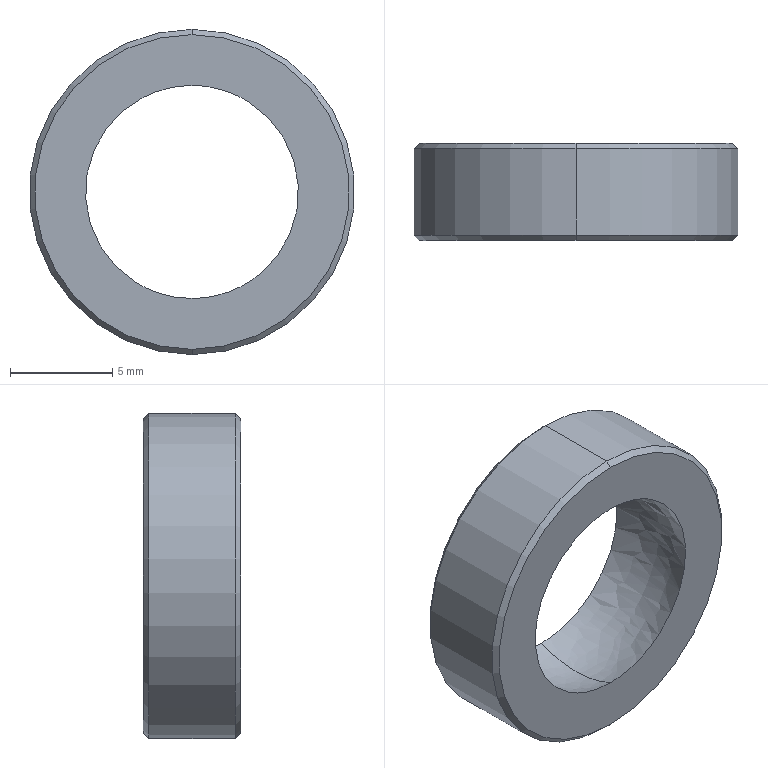Part | SolidWorks | features BaseBody 1 | 1 solid | 10 faces | box 15.875 x 4.75 x 15.875 mm | volume 477.33 mm3 | cone 4 | spline 2 | cylinder 2 | plane 2 | commonest cylinder face diameters 15.875 x2
STEP:
#1=CARTESIAN_POINT('',(0.,-0.000000057,-5.715));
#2=VERTEX_POINT('',#1);
#3=CARTESIAN_POINT('',(0.,2.375,-5.198));
#4=VERTEX_POINT('',#3);
#5=CARTESIAN_POINT('',(0.,0.,0.));
#6=DIRECTION('',(1.,0.,0.));
#7=DIRECTION('',(0.,0.,-1.));
#8=AXIS2_PLACEMENT_3D('',#5,#6,#7);
#9=CIRCLE('',#8,5.715);
#10=EDGE_CURVE('',#2,#4,#9,.T.);
#11=ORIENTED_EDGE('',*,*,#10,.F.);
#12=CARTESIAN_POINT('',(0.,-2.375,-5.198));
#13=VERTEX_POINT('',#12);
#14=CARTESIAN_POINT('',(0.,0.,0.));
#15=DIRECTION('',(-1.,0.,0.));
#16=DIRECTION('',(0.,0.,-1.));
#17=AXIS2_PLACEMENT_3D('',#14,#15,#16);
#18=CIRCLE('',#17,5.715);
#19=EDGE_CURVE('',#2,#13,#18,.T.);
#20=ORIENTED_EDGE('',*,*,#19,.T.);
#21=CARTESIAN_POINT('',(0.000000001,-2.375,5.198));
#22=VERTEX_POINT('',#21);
#23=CARTESIAN_POINT('',(0.,-2.375,-5.198));
#24=CARTESIAN_POINT('',(0.3434,-2.375,-5.198));
#25=CARTESIAN_POINT('',(0.681,-2.375,-5.164));
#26=CARTESIAN_POINT('',(1.179,-2.375,-5.065));
#27=CARTESIAN_POINT('',(1.344,-2.375,-5.024));
#28=CARTESIAN_POINT('',(1.67,-2.375,-4.925));
#29=CARTESIAN_POINT('',(1.833,-2.375,-4.867));
#30=CARTESIAN_POINT('',(2.305,-2.375,-4.672));
#31=CARTESIAN_POINT('',(2.603,-2.375,-4.512));
#32=CARTESIAN_POINT('',(3.168,-2.375,-4.135));
#33=CARTESIAN_POINT('',(3.436,-2.375,-3.915));
#34=CARTESIAN_POINT('',(3.915,-2.375,-3.436));
#35=CARTESIAN_POINT('',(4.131,-2.375,-3.174));
#36=CARTESIAN_POINT('',(4.511,-2.375,-2.606));
#37=CARTESIAN_POINT('',(4.672,-2.375,-2.304));
#38=CARTESIAN_POINT('',(4.931,-2.375,-1.678));
#39=CARTESIAN_POINT('',(5.031,-2.375,-1.351));
#40=CARTESIAN_POINT('',(5.165,-2.375,-0.6797));
#41=CARTESIAN_POINT('',(5.198,-2.375,-0.3425));
#42=CARTESIAN_POINT('',(5.198,-2.375,0.3355));
#43=CARTESIAN_POINT('',(5.165,-2.375,0.6798));
#44=CARTESIAN_POINT('',(5.032,-2.375,1.346));
#45=CARTESIAN_POINT('',(4.934,-2.375,1.67));
#46=CARTESIAN_POINT('',(4.739,-2.375,2.142));
#47=CARTESIAN_POINT('',(4.666,-2.375,2.298));
#48=CARTESIAN_POINT('',(4.505,-2.375,2.599));
#49=CARTESIAN_POINT('',(4.418,-2.375,2.745));
#50=CARTESIAN_POINT('',(4.135,-2.375,3.168));
#51=CARTESIAN_POINT('',(3.921,-2.375,3.43));
#52=CARTESIAN_POINT('',(3.436,-2.375,3.916));
#53=CARTESIAN_POINT('',(3.173,-2.375,4.131));
#54=CARTESIAN_POINT('',(2.751,-2.375,4.414));
#55=CARTESIAN_POINT('',(2.605,-2.375,4.501));
#56=CARTESIAN_POINT('',(2.305,-2.375,4.662));
#57=CARTESIAN_POINT('',(2.149,-2.375,4.736));
#58=CARTESIAN_POINT('',(1.677,-2.375,4.932));
#59=CARTESIAN_POINT('',(1.353,-2.375,5.031));
#60=CARTESIAN_POINT('',(0.687,-2.375,5.164));
#61=CARTESIAN_POINT('',(0.3434,-2.375,5.198));
#62=CARTESIAN_POINT('',(0.000000001,-2.375,5.198));
#63=B_SPLINE_CURVE_WITH_KNOTS('',3,(#23,#24,#25,#26,#27,#28,#29,#30,#31,#32,#33,#34,#35,#36,#37,#38,#39,#40,#41,#42,#43,#44,#45,#46,#47,#48,#49,#50,#51,#52,#53,#54,#55,#56,#57,#58,#59,#60,#61,#62),.UNSPECIFIED.,.F.,.F.,(4,2,2,2,2,2,2,2,2,2,2,2,2,2,2,2,2,2,2,4),(0.01625,0.01726,0.01777,0.01828,0.0193,0.02031,0.02133,0.02234,0.02336,0.02437,0.02539,0.0264,0.02691,0.02742,0.02843,0.02945,0.02996,0.03047,0.03148,0.0325),.UNSPECIFIED.);
#64=EDGE_CURVE('',#13,#22,#63,.T.);
#65=ORIENTED_EDGE('',*,*,#64,.T.);
#66=CARTESIAN_POINT('',(0.,0.000000055,5.715));
#67=VERTEX_POINT('',#66);
#68=CARTESIAN_POINT('',(0.,0.,0.));
#69=DIRECTION('',(-1.,0.,0.));
#70=DIRECTION('',(0.,0.,-1.));
#71=AXIS2_PLACEMENT_3D('',#68,#69,#70);
#72=CIRCLE('',#71,5.715);
#73=EDGE_CURVE('',#22,#67,#72,.T.);
#74=ORIENTED_EDGE('',*,*,#73,.T.);
#75=CARTESIAN_POINT('',(0.,2.375,5.198));
#76=VERTEX_POINT('',#75);
#77=CARTESIAN_POINT('',(0.,0.,0.));
#78=DIRECTION('',(1.,0.,0.));
#79=DIRECTION('',(0.,0.,-1.));
#80=AXIS2_PLACEMENT_3D('',#77,#78,#79);
#81=CIRCLE('',#80,5.715);
#82=EDGE_CURVE('',#76,#67,#81,.T.);
#83=ORIENTED_EDGE('',*,*,#82,.F.);
#84=CARTESIAN_POINT('',(0.,2.375,-5.198));
#85=CARTESIAN_POINT('',(0.3434,2.375,-5.198));
#86=CARTESIAN_POINT('',(0.681,2.375,-5.164));
#87=CARTESIAN_POINT('',(1.179,2.375,-5.065));
#88=CARTESIAN_POINT('',(1.344,2.375,-5.024));
#89=CARTESIAN_POINT('',(1.67,2.375,-4.925));
#90=CARTESIAN_POINT('',(1.833,2.375,-4.867));
#91=CARTESIAN_POINT('',(2.305,2.375,-4.672));
#92=CARTESIAN_POINT('',(2.603,2.375,-4.512));
#93=CARTESIAN_POINT('',(3.168,2.375,-4.135));
#94=CARTESIAN_POINT('',(3.436,2.375,-3.915));
#95=CARTESIAN_POINT('',(3.915,2.375,-3.436));
#96=CARTESIAN_POINT('',(4.131,2.375,-3.174));
#97=CARTESIAN_POINT('',(4.511,2.375,-2.606));
#98=CARTESIAN_POINT('',(4.672,2.375,-2.304));
#99=CARTESIAN_POINT('',(4.931,2.375,-1.678));
#100=CARTESIAN_POINT('',(5.031,2.375,-1.351));
#101=CARTESIAN_POINT('',(5.165,2.375,-0.6797));
#102=CARTESIAN_POINT('',(5.198,2.375,-0.3425));
#103=CARTESIAN_POINT('',(5.198,2.375,0.3355));
#104=CARTESIAN_POINT('',(5.165,2.375,0.6798));
#105=CARTESIAN_POINT('',(5.032,2.375,1.346));
#106=CARTESIAN_POINT('',(4.934,2.375,1.67));
#107=CARTESIAN_POINT('',(4.739,2.375,2.142));
#108=CARTESIAN_POINT('',(4.666,2.375,2.298));
#109=CARTESIAN_POINT('',(4.505,2.375,2.599));
#110=CARTESIAN_POINT('',(4.418,2.375,2.745));
#111=CARTESIAN_POINT('',(4.135,2.375,3.168));
#112=CARTESIAN_POINT('',(3.921,2.375,3.43));
#113=CARTESIAN_POINT('',(3.436,2.375,3.916));
#114=CARTESIAN_POINT('',(3.173,2.375,4.131));
#115=CARTESIAN_POINT('',(2.751,2.375,4.414));
#116=CARTESIAN_POINT('',(2.605,2.375,4.501));
#117=CARTESIAN_POINT('',(2.305,2.375,4.662));
#118=CARTESIAN_POINT('',(2.149,2.375,4.736));
#119=CARTESIAN_POINT('',(1.677,2.375,4.932));
#120=CARTESIAN_POINT('',(1.353,2.375,5.031));
#121=CARTESIAN_POINT('',(0.687,2.375,5.164));
#122=CARTESIAN_POINT('',(0.3434,2.375,5.198));
#123=CARTESIAN_POINT('',(0.,2.375,5.198));
#124=B_SPLINE_CURVE_WITH_KNOTS('',3,(#84,#85,#86,#87,#88,#89,#90,#91,#92,#93,#94,#95,#96,#97,#98,#99,#100,#101,#102,#103,#104,#105,#106,#107,#108,#109,#110,#111,#112,#113,#114,#115,#116,#117,#118,#119,#120,#121,#122,#123),.UNSPECIFIED.,.F.,.F.,(4,2,2,2,2,2,2,2,2,2,2,2,2,2,2,2,2,2,2,4),(0.01625,0.01726,0.01777,0.01828,0.0193,0.02031,0.02133,0.02234,0.02336,0.02437,0.02539,0.0264,0.02691,0.02742,0.02843,0.02945,0.02996,0.03047,0.03148,0.0325),.UNSPECIFIED.);
#125=EDGE_CURVE('',#4,#76,#124,.T.);
#126=ORIENTED_EDGE('',*,*,#125,.F.);
#127=EDGE_LOOP('',(#11,#20,#65,#74,#83,#126));
#128=FACE_OUTER_BOUND('',#127,.T.);
#129=CARTESIAN_POINT('',(0.,0.,-5.715));
#130=CARTESIAN_POINT('',(0.,0.,-5.715));
#131=CARTESIAN_POINT('',(0.,0.,-5.715));
#132=CARTESIAN_POINT('',(0.,0.,-5.715));
#133=CARTESIAN_POINT('',(0.,-11.43,-5.715));
#134=CARTESIAN_POINT('',(22.86,-11.43,-5.715));
#135=CARTESIAN_POINT('',(22.86,11.43,-5.715));
#136=CARTESIAN_POINT('',(0.,11.43,-5.715));
#137=CARTESIAN_POINT('',(0.,-11.43,5.715));
#138=CARTESIAN_POINT('',(22.86,-11.43,5.715));
#139=CARTESIAN_POINT('',(22.86,11.43,5.715));
#140=CARTESIAN_POINT('',(0.,11.43,5.715));
#141=CARTESIAN_POINT('',(0.,0.,5.715));
#142=CARTESIAN_POINT('',(0.,0.,5.715));
#143=CARTESIAN_POINT('',(0.,0.,5.715));
#144=CARTESIAN_POINT('',(0.,0.,5.715));
#145=(BOUNDED_SURFACE()B_SPLINE_SURFACE(3,3,((#129,#130,#131,#132),(#133,#134,#135,#136),(#137,#138,#139,#140),(#141,#142,#143,#144)),.UNSPECIFIED.,.F.,.F.,.F.)B_SPLINE_SURFACE_WITH_KNOTS((4,4),(4,4),(0.,1.),(0.,1.),.UNSPECIFIED.)GEOMETRIC_REPRESENTATION_ITEM()RATIONAL_B_SPLINE_SURFACE(((1.,0.3333,0.3333,1.),(0.3333,0.1111,0.1111,0.3333),(0.3333,0.1111,0.1111,0.3333),(1.,0.3333,0.3333,1.)))REPRESENTATION_ITEM('')SURFACE());
#146=ADVANCED_FACE('',(#128),#145,.T.);
#147=CARTESIAN_POINT('',(0.,2.375,7.684));
#148=VERTEX_POINT('',#147);
#149=CARTESIAN_POINT('',(0.,2.375,-7.684));
#150=VERTEX_POINT('',#149);
#151=CARTESIAN_POINT('',(0.,2.375,0.));
#152=DIRECTION('',(0.,1.,0.));
#153=DIRECTION('',(0.,0.,-1.));
#154=AXIS2_PLACEMENT_3D('',#151,#152,#153);
#155=CIRCLE('',#154,7.684);
#156=EDGE_CURVE('',#148,#150,#155,.T.);
#157=ORIENTED_EDGE('',*,*,#156,.F.);
#158=CARTESIAN_POINT('',(0.,2.121,7.938));
#159=VERTEX_POINT('',#158);
#160=CARTESIAN_POINT('',(0.,2.375,7.683));
#161=DIRECTION('',(0.,-0.7071,0.7071));
#162=VECTOR('',#161,1000.);
#163=LINE('',#160,#162);
#164=EDGE_CURVE('',#148,#159,#163,.T.);
#165=ORIENTED_EDGE('',*,*,#164,.T.);
#166=CARTESIAN_POINT('',(0.,2.121,-7.938));
#167=VERTEX_POINT('',#166);
#168=CARTESIAN_POINT('',(0.,2.121,0.));
#169=DIRECTION('',(0.,-1.,0.));
#170=DIRECTION('',(0.,0.,-1.));
#171=AXIS2_PLACEMENT_3D('',#168,#169,#170);
#172=CIRCLE('',#171,7.938);
#173=EDGE_CURVE('',#167,#159,#172,.T.);
#174=ORIENTED_EDGE('',*,*,#173,.F.);
#175=CARTESIAN_POINT('',(0.,2.375,-7.683));
#176=DIRECTION('',(0.,-0.7071,-0.7071));
#177=VECTOR('',#176,1000.);
#178=LINE('',#175,#177);
#179=EDGE_CURVE('',#150,#167,#178,.T.);
#180=ORIENTED_EDGE('',*,*,#179,.F.);
#181=EDGE_LOOP('',(#157,#165,#174,#180));
#182=FACE_OUTER_BOUND('',#181,.T.);
#183=CARTESIAN_POINT('',(0.,2.375,0.));
#184=DIRECTION('',(0.,-1.,0.));
#185=DIRECTION('',(0.,0.,-1.));
#186=AXIS2_PLACEMENT_3D('',#183,#184,#185);
#187=CONICAL_SURFACE('',#186,7.683,0.7854);
#188=ADVANCED_FACE('',(#182),#187,.T.);
#189=ORIENTED_EDGE('',*,*,#173,.T.);
#190=CARTESIAN_POINT('',(0.,-2.121,7.938));
#191=VERTEX_POINT('',#190);
#192=CARTESIAN_POINT('',(0.,2.121,7.938));
#193=DIRECTION('',(0.,-1.,0.));
#194=VECTOR('',#193,1000.);
#195=LINE('',#192,#194);
#196=EDGE_CURVE('',#159,#191,#195,.T.);
#197=ORIENTED_EDGE('',*,*,#196,.T.);
#198=CARTESIAN_POINT('',(0.,-2.121,-7.938));
#199=VERTEX_POINT('',#198);
#200=CARTESIAN_POINT('',(0.,-2.121,0.));
#201=DIRECTION('',(0.,-1.,0.));
#202=DIRECTION('',(0.,0.,-1.));
#203=AXIS2_PLACEMENT_3D('',#200,#201,#202);
#204=CIRCLE('',#203,7.938);
#205=EDGE_CURVE('',#199,#191,#204,.T.);
#206=ORIENTED_EDGE('',*,*,#205,.F.);
#207=CARTESIAN_POINT('',(0.,2.121,-7.938));
#208=DIRECTION('',(0.,-1.,0.));
#209=VECTOR('',#208,1000.);
#210=LINE('',#207,#209);
#211=EDGE_CURVE('',#167,#199,#210,.T.);
#212=ORIENTED_EDGE('',*,*,#211,.F.);
#213=EDGE_LOOP('',(#189,#197,#206,#212));
#214=FACE_OUTER_BOUND('',#213,.T.);
#215=CARTESIAN_POINT('',(0.,2.121,0.));
#216=DIRECTION('',(0.,-1.,0.));
#217=DIRECTION('',(0.,0.,-1.));
#218=AXIS2_PLACEMENT_3D('',#215,#216,#217);
#219=CYLINDRICAL_SURFACE('',#218,7.938);
#220=ADVANCED_FACE('',(#214),#219,.T.);
#221=CARTESIAN_POINT('',(0.,-2.375,-7.684));
#222=VERTEX_POINT('',#221);
#223=CARTESIAN_POINT('',(0.,-2.375,7.684));
#224=VERTEX_POINT('',#223);
#225=CARTESIAN_POINT('',(0.,-2.375,0.));
#226=DIRECTION('',(0.,-1.,0.));
#227=DIRECTION('',(0.,0.,1.));
#228=AXIS2_PLACEMENT_3D('',#225,#226,#227);
#229=CIRCLE('',#228,7.684);
#230=EDGE_CURVE('',#222,#224,#229,.T.);
#231=ORIENTED_EDGE('',*,*,#230,.F.);
#232=CARTESIAN_POINT('',(0.,-2.375,-7.683));
#233=DIRECTION('',(0.,0.7071,-0.7071));
#234=VECTOR('',#233,1000.);
#235=LINE('',#232,#234);
#236=EDGE_CURVE('',#222,#199,#235,.T.);
#237=ORIENTED_EDGE('',*,*,#236,.T.);
#238=ORIENTED_EDGE('',*,*,#205,.T.);
#239=CARTESIAN_POINT('',(0.,-2.375,7.683));
#240=DIRECTION('',(0.,0.7071,0.7071));
#241=VECTOR('',#240,1000.);
#242=LINE('',#239,#241);
#243=EDGE_CURVE('',#224,#191,#242,.T.);
#244=ORIENTED_EDGE('',*,*,#243,.F.);
#245=EDGE_LOOP('',(#231,#237,#238,#244));
#246=FACE_OUTER_BOUND('',#245,.T.);
#247=CARTESIAN_POINT('',(0.,-2.375,0.));
#248=DIRECTION('',(0.,1.,0.));
#249=DIRECTION('',(0.,0.,1.));
#250=AXIS2_PLACEMENT_3D('',#247,#248,#249);
#251=CONICAL_SURFACE('',#250,7.683,0.7854);
#252=ADVANCED_FACE('',(#246),#251,.T.);
#253=ORIENTED_EDGE('',*,*,#164,.F.);
#254=CARTESIAN_POINT('',(0.,2.375,0.));
#255=DIRECTION('',(0.,1.,0.));
#256=DIRECTION('',(0.,0.,-1.));
#257=AXIS2_PLACEMENT_3D('',#254,#255,#256);
#258=CIRCLE('',#257,7.684);
#259=EDGE_CURVE('',#150,#148,#258,.T.);
#260=ORIENTED_EDGE('',*,*,#259,.F.);
#261=ORIENTED_EDGE('',*,*,#179,.T.);
#262=CARTESIAN_POINT('',(0.,2.121,0.));
#263=DIRECTION('',(0.,-1.,0.));
#264=DIRECTION('',(0.,0.,-1.));
#265=AXIS2_PLACEMENT_3D('',#262,#263,#264);
#266=CIRCLE('',#265,7.938);
#267=EDGE_CURVE('',#159,#167,#266,.T.);
#268=ORIENTED_EDGE('',*,*,#267,.F.);
#269=EDGE_LOOP('',(#253,#260,#261,#268));
#270=FACE_OUTER_BOUND('',#269,.T.);
#271=CARTESIAN_POINT('',(0.,2.375,0.));
#272=DIRECTION('',(0.,-1.,0.));
#273=DIRECTION('',(0.,0.,-1.));
#274=AXIS2_PLACEMENT_3D('',#271,#272,#273);
#275=CONICAL_SURFACE('',#274,7.683,0.7854);
#276=ADVANCED_FACE('',(#270),#275,.T.);
#277=CARTESIAN_POINT('',(0.,2.375,5.198));
#278=CARTESIAN_POINT('',(-0.3434,2.375,5.198));
#279=CARTESIAN_POINT('',(-0.681,2.375,5.164));
#280=CARTESIAN_POINT('',(-1.179,2.375,5.065));
#281=CARTESIAN_POINT('',(-1.344,2.375,5.024));
#282=CARTESIAN_POINT('',(-1.67,2.375,4.925));
#283=CARTESIAN_POINT('',(-1.833,2.375,4.867));
#284=CARTESIAN_POINT('',(-2.305,2.375,4.672));
#285=CARTESIAN_POINT('',(-2.603,2.375,4.512));
#286=CARTESIAN_POINT('',(-3.168,2.375,4.135));
#287=CARTESIAN_POINT('',(-3.436,2.375,3.915));
#288=CARTESIAN_POINT('',(-3.915,2.375,3.436));
#289=CARTESIAN_POINT('',(-4.131,2.375,3.174));
#290=CARTESIAN_POINT('',(-4.511,2.375,2.606));
#291=CARTESIAN_POINT('',(-4.672,2.375,2.304));
#292=CARTESIAN_POINT('',(-4.931,2.375,1.678));
#293=CARTESIAN_POINT('',(-5.031,2.375,1.351));
#294=CARTESIAN_POINT('',(-5.165,2.375,0.6797));
#295=CARTESIAN_POINT('',(-5.198,2.375,0.3425));
#296=CARTESIAN_POINT('',(-5.198,2.375,-0.3355));
#297=CARTESIAN_POINT('',(-5.165,2.375,-0.6798));
#298=CARTESIAN_POINT('',(-5.032,2.375,-1.346));
#299=CARTESIAN_POINT('',(-4.934,2.375,-1.67));
#300=CARTESIAN_POINT('',(-4.739,2.375,-2.142));
#301=CARTESIAN_POINT('',(-4.666,2.375,-2.298));
#302=CARTESIAN_POINT('',(-4.505,2.375,-2.599));
#303=CARTESIAN_POINT('',(-4.418,2.375,-2.745));
#304=CARTESIAN_POINT('',(-4.135,2.375,-3.168));
#305=CARTESIAN_POINT('',(-3.921,2.375,-3.43));
#306=CARTESIAN_POINT('',(-3.436,2.375,-3.916));
#307=CARTESIAN_POINT('',(-3.173,2.375,-4.131));
#308=CARTESIAN_POINT('',(-2.751,2.375,-4.414));
#309=CARTESIAN_POINT('',(-2.605,2.375,-4.501));
#310=CARTESIAN_POINT('',(-2.305,2.375,-4.662));
#311=CARTESIAN_POINT('',(-2.149,2.375,-4.736));
#312=CARTESIAN_POINT('',(-1.677,2.375,-4.932));
#313=CARTESIAN_POINT('',(-1.353,2.375,-5.031));
#314=CARTESIAN_POINT('',(-0.687,2.375,-5.164));
#315=CARTESIAN_POINT('',(-0.3434,2.375,-5.198));
#316=CARTESIAN_POINT('',(0.,2.375,-5.198));
#317=B_SPLINE_CURVE_WITH_KNOTS('',3,(#277,#278,#279,#280,#281,#282,#283,#284,#285,#286,#287,#288,#289,#290,#291,#292,#293,#294,#295,#296,#297,#298,#299,#300,#301,#302,#303,#304,#305,#306,#307,#308,#309,#310,#311,#312,#313,#314,#315,#316),.UNSPECIFIED.,.F.,.F.,(4,2,2,2,2,2,2,2,2,2,2,2,2,2,2,2,2,2,2,4),(0.,0.001016,0.001523,0.002031,0.003047,0.004062,0.005078,0.006093,0.007109,0.008124,0.00914,0.01016,0.01066,0.01117,0.01219,0.0132,0.01371,0.01422,0.01523,0.01625),.UNSPECIFIED.);
#318=EDGE_CURVE('',#76,#4,#317,.T.);
#319=ORIENTED_EDGE('',*,*,#318,.T.);
#320=ORIENTED_EDGE('',*,*,#125,.T.);
#321=EDGE_LOOP('',(#319,#320));
#322=FACE_BOUND('',#321,.T.);
#323=ORIENTED_EDGE('',*,*,#259,.T.);
#324=ORIENTED_EDGE('',*,*,#156,.T.);
#325=EDGE_LOOP('',(#323,#324));
#326=FACE_OUTER_BOUND('',#325,.T.);
#327=CARTESIAN_POINT('',(-7.776,2.375,-7.776));
#328=DIRECTION('',(0.,1.,0.));
#329=DIRECTION('',(0.,0.,1.));
#330=AXIS2_PLACEMENT_3D('',#327,#328,#329);
#331=PLANE('',#330);
#332=ADVANCED_FACE('',(#322,#326),#331,.T.);
#333=ORIENTED_EDGE('',*,*,#196,.F.);
#334=ORIENTED_EDGE('',*,*,#267,.T.);
#335=ORIENTED_EDGE('',*,*,#211,.T.);
#336=CARTESIAN_POINT('',(0.,-2.121,0.));
#337=DIRECTION('',(0.,-1.,0.));
#338=DIRECTION('',(0.,0.,-1.));
#339=AXIS2_PLACEMENT_3D('',#336,#337,#338);
#340=CIRCLE('',#339,7.938);
#341=EDGE_CURVE('',#191,#199,#340,.T.);
#342=ORIENTED_EDGE('',*,*,#341,.F.);
#343=EDGE_LOOP('',(#333,#334,#335,#342));
#344=FACE_OUTER_BOUND('',#343,.T.);
#345=CARTESIAN_POINT('',(0.,2.121,0.));
#346=DIRECTION('',(0.,-1.,0.));
#347=DIRECTION('',(0.,0.,-1.));
#348=AXIS2_PLACEMENT_3D('',#345,#346,#347);
#349=CYLINDRICAL_SURFACE('',#348,7.938);
#350=ADVANCED_FACE('',(#344),#349,.T.);
#351=ORIENTED_EDGE('',*,*,#19,.F.);
#352=ORIENTED_EDGE('',*,*,#10,.T.);
#353=ORIENTED_EDGE('',*,*,#318,.F.);
#354=ORIENTED_EDGE('',*,*,#82,.T.);
#355=ORIENTED_EDGE('',*,*,#73,.F.);
#356=CARTESIAN_POINT('',(0.000000001,-2.375,5.198));
#357=CARTESIAN_POINT('',(-0.3434,-2.375,5.198));
#358=CARTESIAN_POINT('',(-0.681,-2.375,5.164));
#359=CARTESIAN_POINT('',(-1.179,-2.375,5.065));
#360=CARTESIAN_POINT('',(-1.344,-2.375,5.024));
#361=CARTESIAN_POINT('',(-1.67,-2.375,4.925));
#362=CARTESIAN_POINT('',(-1.833,-2.375,4.867));
#363=CARTESIAN_POINT('',(-2.305,-2.375,4.672));
#364=CARTESIAN_POINT('',(-2.603,-2.375,4.512));
#365=CARTESIAN_POINT('',(-3.168,-2.375,4.135));
#366=CARTESIAN_POINT('',(-3.436,-2.375,3.915));
#367=CARTESIAN_POINT('',(-3.915,-2.375,3.436));
#368=CARTESIAN_POINT('',(-4.131,-2.375,3.174));
#369=CARTESIAN_POINT('',(-4.511,-2.375,2.606));
#370=CARTESIAN_POINT('',(-4.672,-2.375,2.304));
#371=CARTESIAN_POINT('',(-4.931,-2.375,1.678));
#372=CARTESIAN_POINT('',(-5.031,-2.375,1.351));
#373=CARTESIAN_POINT('',(-5.165,-2.375,0.6797));
#374=CARTESIAN_POINT('',(-5.198,-2.375,0.3425));
#375=CARTESIAN_POINT('',(-5.198,-2.375,-0.3355));
#376=CARTESIAN_POINT('',(-5.165,-2.375,-0.6798));
#377=CARTESIAN_POINT('',(-5.032,-2.375,-1.346));
#378=CARTESIAN_POINT('',(-4.934,-2.375,-1.67));
#379=CARTESIAN_POINT('',(-4.739,-2.375,-2.142));
#380=CARTESIAN_POINT('',(-4.666,-2.375,-2.298));
#381=CARTESIAN_POINT('',(-4.505,-2.375,-2.599));
#382=CARTESIAN_POINT('',(-4.418,-2.375,-2.745));
#383=CARTESIAN_POINT('',(-4.135,-2.375,-3.168));
#384=CARTESIAN_POINT('',(-3.921,-2.375,-3.43));
#385=CARTESIAN_POINT('',(-3.436,-2.375,-3.916));
#386=CARTESIAN_POINT('',(-3.173,-2.375,-4.131));
#387=CARTESIAN_POINT('',(-2.751,-2.375,-4.414));
#388=CARTESIAN_POINT('',(-2.605,-2.375,-4.501));
#389=CARTESIAN_POINT('',(-2.305,-2.375,-4.662));
#390=CARTESIAN_POINT('',(-2.149,-2.375,-4.736));
#391=CARTESIAN_POINT('',(-1.677,-2.375,-4.932));
#392=CARTESIAN_POINT('',(-1.353,-2.375,-5.031));
#393=CARTESIAN_POINT('',(-0.687,-2.375,-5.164));
#394=CARTESIAN_POINT('',(-0.3434,-2.375,-5.198));
#395=CARTESIAN_POINT('',(0.,-2.375,-5.198));
#396=B_SPLINE_CURVE_WITH_KNOTS('',3,(#356,#357,#358,#359,#360,#361,#362,#363,#364,#365,#366,#367,#368,#369,#370,#371,#372,#373,#374,#375,#376,#377,#378,#379,#380,#381,#382,#383,#384,#385,#386,#387,#388,#389,#390,#391,#392,#393,#394,#395),.UNSPECIFIED.,.F.,.F.,(4,2,2,2,2,2,2,2,2,2,2,2,2,2,2,2,2,2,2,4),(0.,0.001016,0.001523,0.002031,0.003047,0.004062,0.005078,0.006093,0.007109,0.008124,0.00914,0.01016,0.01066,0.01117,0.01219,0.0132,0.01371,0.01422,0.01523,0.01625),.UNSPECIFIED.);
#397=EDGE_CURVE('',#22,#13,#396,.T.);
#398=ORIENTED_EDGE('',*,*,#397,.T.);
#399=EDGE_LOOP('',(#351,#352,#353,#354,#355,#398));
#400=FACE_OUTER_BOUND('',#399,.T.);
#401=CARTESIAN_POINT('',(0.,0.,-5.715));
#402=CARTESIAN_POINT('',(0.,0.,-5.715));
#403=CARTESIAN_POINT('',(0.,0.,-5.715));
#404=CARTESIAN_POINT('',(0.,0.,-5.715));
#405=CARTESIAN_POINT('',(0.,0.,-5.715));
#406=CARTESIAN_POINT('',(0.,0.,-5.715));
#407=CARTESIAN_POINT('',(0.,0.,-5.715));
#408=CARTESIAN_POINT('',(0.,11.43,-5.715));
#409=CARTESIAN_POINT('',(-6.696,11.43,-5.715));
#410=CARTESIAN_POINT('',(-11.43,6.696,-5.715));
#411=CARTESIAN_POINT('',(-11.43,-0.000000001,-5.715));
#412=CARTESIAN_POINT('',(-11.43,-6.696,-5.715));
#413=CARTESIAN_POINT('',(-6.696,-11.43,-5.715));
#414=CARTESIAN_POINT('',(0.000000003,-11.43,-5.715));
#415=CARTESIAN_POINT('',(0.,11.43,5.715));
#416=CARTESIAN_POINT('',(-6.696,11.43,5.715));
#417=CARTESIAN_POINT('',(-11.43,6.696,5.715));
#418=CARTESIAN_POINT('',(-11.43,-0.000000001,5.715));
#419=CARTESIAN_POINT('',(-11.43,-6.696,5.715));
#420=CARTESIAN_POINT('',(-6.696,-11.43,5.715));
#421=CARTESIAN_POINT('',(0.000000003,-11.43,5.715));
#422=CARTESIAN_POINT('',(0.,0.,5.715));
#423=CARTESIAN_POINT('',(0.,0.,5.715));
#424=CARTESIAN_POINT('',(0.,0.,5.715));
#425=CARTESIAN_POINT('',(0.,0.,5.715));
#426=CARTESIAN_POINT('',(0.,0.,5.715));
#427=CARTESIAN_POINT('',(0.,0.,5.715));
#428=CARTESIAN_POINT('',(0.,0.,5.715));
#429=(BOUNDED_SURFACE()B_SPLINE_SURFACE(3,3,((#401,#402,#403,#404,#405,#406,#407),(#408,#409,#410,#411,#412,#413,#414),(#415,#416,#417,#418,#419,#420,#421),(#422,#423,#424,#425,#426,#427,#428)),.UNSPECIFIED.,.F.,.F.,.F.)B_SPLINE_SURFACE_WITH_KNOTS((4,4),(4,3,4),(0.,1.),(0.,0.5,1.),.UNSPECIFIED.)GEOMETRIC_REPRESENTATION_ITEM()RATIONAL_B_SPLINE_SURFACE(((1.,0.8047,0.8047,1.,0.8047,0.8047,1.),(0.3333,0.2682,0.2682,0.3333,0.2682,0.2682,0.3333),(0.3333,0.2682,0.2682,0.3333,0.2682,0.2682,0.3333),(1.,0.8047,0.8047,1.,0.8047,0.8047,1.)))REPRESENTATION_ITEM('')SURFACE());
#430=ADVANCED_FACE('',(#400),#429,.T.);
#431=ORIENTED_EDGE('',*,*,#236,.F.);
#432=CARTESIAN_POINT('',(0.,-2.375,0.));
#433=DIRECTION('',(0.,-1.,0.));
#434=DIRECTION('',(0.,0.,1.));
#435=AXIS2_PLACEMENT_3D('',#432,#433,#434);
#436=CIRCLE('',#435,7.684);
#437=EDGE_CURVE('',#224,#222,#436,.T.);
#438=ORIENTED_EDGE('',*,*,#437,.F.);
#439=ORIENTED_EDGE('',*,*,#243,.T.);
#440=ORIENTED_EDGE('',*,*,#341,.T.);
#441=EDGE_LOOP('',(#431,#438,#439,#440));
#442=FACE_OUTER_BOUND('',#441,.T.);
#443=CARTESIAN_POINT('',(0.,-2.375,0.));
#444=DIRECTION('',(0.,1.,0.));
#445=DIRECTION('',(0.,0.,1.));
#446=AXIS2_PLACEMENT_3D('',#443,#444,#445);
#447=CONICAL_SURFACE('',#446,7.683,0.7854);
#448=ADVANCED_FACE('',(#442),#447,.T.);
#449=ORIENTED_EDGE('',*,*,#397,.F.);
#450=ORIENTED_EDGE('',*,*,#64,.F.);
#451=EDGE_LOOP('',(#449,#450));
#452=FACE_BOUND('',#451,.T.);
#453=ORIENTED_EDGE('',*,*,#437,.T.);
#454=ORIENTED_EDGE('',*,*,#230,.T.);
#455=EDGE_LOOP('',(#453,#454));
#456=FACE_OUTER_BOUND('',#455,.T.);
#457=CARTESIAN_POINT('',(-7.776,-2.375,-7.776));
#458=DIRECTION('',(0.,1.,0.));
#459=DIRECTION('',(0.,0.,1.));
#460=AXIS2_PLACEMENT_3D('',#457,#458,#459);
#461=PLANE('',#460);
#462=ADVANCED_FACE('',(#452,#456),#461,.F.);
#463=CLOSED_SHELL('',(#146,#188,#220,#252,#276,#332,#350,#430,#448,#462));
#464=MANIFOLD_SOLID_BREP('',#463);
#465=CARTESIAN_POINT('',(0.,0.,0.));
#466=DIRECTION('',(0.,0.,1.));
#467=DIRECTION('',(1.,0.,0.));
#468=AXIS2_PLACEMENT_3D('',#465,#466,#467);
#469=(LENGTH_UNIT()NAMED_UNIT(*)SI_UNIT(.MILLI.,.METRE.));
#470=UNCERTAINTY_MEASURE_WITH_UNIT(LENGTH_MEASURE(0.00001),#469,'','');
#471=(NAMED_UNIT(*)PLANE_ANGLE_UNIT()SI_UNIT($,.RADIAN.));
#472=(NAMED_UNIT(*)SI_UNIT($,.STERADIAN.)SOLID_ANGLE_UNIT());
#473=(GEOMETRIC_REPRESENTATION_CONTEXT(3)GLOBAL_UNCERTAINTY_ASSIGNED_CONTEXT((#470))GLOBAL_UNIT_ASSIGNED_CONTEXT((#469,#471,#472))REPRESENTATION_CONTEXT('',''));
#474=ADVANCED_BREP_SHAPE_REPRESENTATION('',(#464,#468),#473);